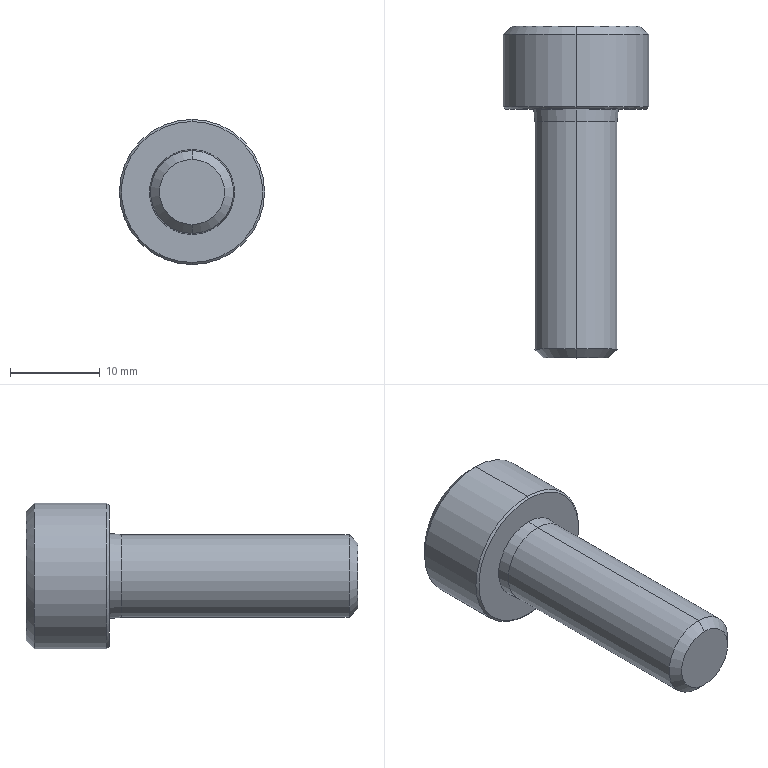Part | SolidWorks | features BaseBody 1 | 1 solid | 36 faces | box 16.154 x 36.923 x 16.154 mm | volume 3494 mm3 | cone 17 | plane 15 | cylinder 4 | commonest cylinder face diameters 9.231 x2 16.154 x2
STEP:
#1=CARTESIAN_POINT('',(-35.061,271.722,102.846));
#2=VERTEX_POINT('',#1);
#3=CARTESIAN_POINT('',(-35.061,271.722,93.615));
#4=VERTEX_POINT('',#3);
#5=CARTESIAN_POINT('',(-35.061,271.722,98.231));
#6=DIRECTION('',(0.,1.,0.));
#7=DIRECTION('',(0.,0.,1.));
#8=AXIS2_PLACEMENT_3D('',#5,#6,#7);
#9=CIRCLE('',#8,4.615);
#10=EDGE_CURVE('',#2,#4,#9,.T.);
#11=ORIENTED_EDGE('',*,*,#10,.T.);
#12=CARTESIAN_POINT('',(-35.061,297.039,93.615));
#13=VERTEX_POINT('',#12);
#14=CARTESIAN_POINT('',(-35.061,270.731,93.615));
#15=DIRECTION('',(0.,1.,0.));
#16=VECTOR('',#15,1000.);
#17=LINE('',#14,#16);
#18=EDGE_CURVE('',#4,#13,#17,.T.);
#19=ORIENTED_EDGE('',*,*,#18,.T.);
#20=CARTESIAN_POINT('',(-35.061,297.039,102.846));
#21=VERTEX_POINT('',#20);
#22=CARTESIAN_POINT('',(-35.061,297.039,98.231));
#23=DIRECTION('',(0.,-1.,0.));
#24=DIRECTION('',(0.,0.,1.));
#25=AXIS2_PLACEMENT_3D('',#22,#23,#24);
#26=CIRCLE('',#25,4.615);
#27=EDGE_CURVE('',#13,#21,#26,.T.);
#28=ORIENTED_EDGE('',*,*,#27,.T.);
#29=CARTESIAN_POINT('',(-35.061,270.731,102.846));
#30=DIRECTION('',(0.,1.,0.));
#31=VECTOR('',#30,1000.);
#32=LINE('',#29,#31);
#33=EDGE_CURVE('',#2,#21,#32,.T.);
#34=ORIENTED_EDGE('',*,*,#33,.F.);
#35=EDGE_LOOP('',(#11,#19,#28,#34));
#36=FACE_OUTER_BOUND('',#35,.T.);
#37=CARTESIAN_POINT('',(-35.061,270.731,98.231));
#38=DIRECTION('',(0.,1.,0.));
#39=DIRECTION('',(0.,0.,1.));
#40=AXIS2_PLACEMENT_3D('',#37,#38,#39);
#41=CYLINDRICAL_SURFACE('',#40,4.615);
#42=ADVANCED_FACE('',(#36),#41,.T.);
#43=CARTESIAN_POINT('',(-35.061,270.731,101.855));
#44=VERTEX_POINT('',#43);
#45=CARTESIAN_POINT('',(-35.061,270.731,94.607));
#46=VERTEX_POINT('',#45);
#47=CARTESIAN_POINT('',(-35.061,270.731,98.231));
#48=DIRECTION('',(0.,1.,0.));
#49=DIRECTION('',(0.,0.,1.));
#50=AXIS2_PLACEMENT_3D('',#47,#48,#49);
#51=CIRCLE('',#50,3.624);
#52=EDGE_CURVE('',#44,#46,#51,.T.);
#53=ORIENTED_EDGE('',*,*,#52,.T.);
#54=CARTESIAN_POINT('',(-35.061,271.722,93.615));
#55=DIRECTION('',(0.,0.7071,-0.7071));
#56=VECTOR('',#55,1000.);
#57=LINE('',#54,#56);
#58=EDGE_CURVE('',#46,#4,#57,.T.);
#59=ORIENTED_EDGE('',*,*,#58,.T.);
#60=ORIENTED_EDGE('',*,*,#10,.F.);
#61=CARTESIAN_POINT('',(-35.061,271.722,102.846));
#62=DIRECTION('',(0.,0.7071,0.7071));
#63=VECTOR('',#62,1000.);
#64=LINE('',#61,#63);
#65=EDGE_CURVE('',#44,#2,#64,.T.);
#66=ORIENTED_EDGE('',*,*,#65,.F.);
#67=EDGE_LOOP('',(#53,#59,#60,#66));
#68=FACE_OUTER_BOUND('',#67,.T.);
#69=CARTESIAN_POINT('',(-35.061,271.722,98.231));
#70=DIRECTION('',(0.,1.,0.));
#71=DIRECTION('',(0.,0.,1.));
#72=AXIS2_PLACEMENT_3D('',#69,#70,#71);
#73=CONICAL_SURFACE('',#72,4.615,0.7854);
#74=ADVANCED_FACE('',(#68),#73,.T.);
#75=ORIENTED_EDGE('',*,*,#27,.F.);
#76=CARTESIAN_POINT('',(-35.061,298.423,93.5));
#77=VERTEX_POINT('',#76);
#78=CARTESIAN_POINT('',(-35.061,298.423,93.5));
#79=DIRECTION('',(0.,0.9965,-0.08305));
#80=VECTOR('',#79,1000.);
#81=LINE('',#78,#80);
#82=EDGE_CURVE('',#13,#77,#81,.T.);
#83=ORIENTED_EDGE('',*,*,#82,.T.);
#84=CARTESIAN_POINT('',(-35.061,298.423,102.962));
#85=VERTEX_POINT('',#84);
#86=CARTESIAN_POINT('',(-35.061,298.423,98.231));
#87=DIRECTION('',(0.,-1.,0.));
#88=DIRECTION('',(0.,0.,1.));
#89=AXIS2_PLACEMENT_3D('',#86,#87,#88);
#90=CIRCLE('',#89,4.731);
#91=EDGE_CURVE('',#77,#85,#90,.T.);
#92=ORIENTED_EDGE('',*,*,#91,.T.);
#93=CARTESIAN_POINT('',(-35.061,298.423,102.962));
#94=DIRECTION('',(0.,0.9965,0.08305));
#95=VECTOR('',#94,1000.);
#96=LINE('',#93,#95);
#97=EDGE_CURVE('',#21,#85,#96,.T.);
#98=ORIENTED_EDGE('',*,*,#97,.F.);
#99=EDGE_LOOP('',(#75,#83,#92,#98));
#100=FACE_OUTER_BOUND('',#99,.T.);
#101=CARTESIAN_POINT('',(-35.061,298.423,98.231));
#102=DIRECTION('',(0.,1.,0.));
#103=DIRECTION('',(0.,0.,1.));
#104=AXIS2_PLACEMENT_3D('',#101,#102,#103);
#105=CONICAL_SURFACE('',#104,4.731,0.08314);
#106=ADVANCED_FACE('',(#100),#105,.T.);
#107=CARTESIAN_POINT('',(-35.061,298.423,106.077));
#108=VERTEX_POINT('',#107);
#109=CARTESIAN_POINT('',(-35.061,298.423,90.385));
#110=VERTEX_POINT('',#109);
#111=CARTESIAN_POINT('',(-35.061,298.423,98.231));
#112=DIRECTION('',(0.,1.,0.));
#113=DIRECTION('',(0.,0.,1.));
#114=AXIS2_PLACEMENT_3D('',#111,#112,#113);
#115=CIRCLE('',#114,7.846);
#116=EDGE_CURVE('',#108,#110,#115,.T.);
#117=ORIENTED_EDGE('',*,*,#116,.T.);
#118=CARTESIAN_POINT('',(-35.061,298.654,90.154));
#119=VERTEX_POINT('',#118);
#120=CARTESIAN_POINT('',(-35.061,298.654,90.154));
#121=DIRECTION('',(0.,0.7071,-0.7071));
#122=VECTOR('',#121,1000.);
#123=LINE('',#120,#122);
#124=EDGE_CURVE('',#110,#119,#123,.T.);
#125=ORIENTED_EDGE('',*,*,#124,.T.);
#126=CARTESIAN_POINT('',(-35.061,298.654,106.308));
#127=VERTEX_POINT('',#126);
#128=CARTESIAN_POINT('',(-35.061,298.654,98.231));
#129=DIRECTION('',(0.,-1.,0.));
#130=DIRECTION('',(-1.,0.,0.));
#131=AXIS2_PLACEMENT_3D('',#128,#129,#130);
#132=CIRCLE('',#131,8.077);
#133=EDGE_CURVE('',#119,#127,#132,.T.);
#134=ORIENTED_EDGE('',*,*,#133,.T.);
#135=CARTESIAN_POINT('',(-35.061,298.654,106.308));
#136=DIRECTION('',(0.,0.7071,0.7071));
#137=VECTOR('',#136,1000.);
#138=LINE('',#135,#137);
#139=EDGE_CURVE('',#108,#127,#138,.T.);
#140=ORIENTED_EDGE('',*,*,#139,.F.);
#141=EDGE_LOOP('',(#117,#125,#134,#140));
#142=FACE_OUTER_BOUND('',#141,.T.);
#143=CARTESIAN_POINT('',(-35.061,298.654,98.231));
#144=DIRECTION('',(0.,1.,0.));
#145=DIRECTION('',(0.,0.,1.));
#146=AXIS2_PLACEMENT_3D('',#143,#144,#145);
#147=CONICAL_SURFACE('',#146,8.077,0.7854);
#148=ADVANCED_FACE('',(#142),#147,.T.);
#149=ORIENTED_EDGE('',*,*,#133,.F.);
#150=CARTESIAN_POINT('',(-35.061,306.731,90.154));
#151=VERTEX_POINT('',#150);
#152=CARTESIAN_POINT('',(-35.061,270.731,90.154));
#153=DIRECTION('',(0.,1.,0.));
#154=VECTOR('',#153,1000.);
#155=LINE('',#152,#154);
#156=EDGE_CURVE('',#119,#151,#155,.T.);
#157=ORIENTED_EDGE('',*,*,#156,.T.);
#158=CARTESIAN_POINT('',(-35.061,306.731,106.308));
#159=VERTEX_POINT('',#158);
#160=CARTESIAN_POINT('',(-35.061,306.731,98.231));
#161=DIRECTION('',(0.,-1.,0.));
#162=DIRECTION('',(0.,0.,1.));
#163=AXIS2_PLACEMENT_3D('',#160,#161,#162);
#164=CIRCLE('',#163,8.077);
#165=EDGE_CURVE('',#151,#159,#164,.T.);
#166=ORIENTED_EDGE('',*,*,#165,.T.);
#167=CARTESIAN_POINT('',(-35.061,270.731,106.308));
#168=DIRECTION('',(0.,1.,0.));
#169=VECTOR('',#168,1000.);
#170=LINE('',#167,#169);
#171=EDGE_CURVE('',#127,#159,#170,.T.);
#172=ORIENTED_EDGE('',*,*,#171,.F.);
#173=EDGE_LOOP('',(#149,#157,#166,#172));
#174=FACE_OUTER_BOUND('',#173,.T.);
#175=CARTESIAN_POINT('',(-35.061,270.731,98.231));
#176=DIRECTION('',(0.,1.,0.));
#177=DIRECTION('',(0.,0.,1.));
#178=AXIS2_PLACEMENT_3D('',#175,#176,#177);
#179=CYLINDRICAL_SURFACE('',#178,8.077);
#180=ADVANCED_FACE('',(#174),#179,.T.);
#181=CARTESIAN_POINT('',(-35.061,307.654,91.077));
#182=VERTEX_POINT('',#181);
#183=CARTESIAN_POINT('',(-35.061,307.654,105.385));
#184=VERTEX_POINT('',#183);
#185=CARTESIAN_POINT('',(-35.061,307.654,98.231));
#186=DIRECTION('',(0.,-1.,0.));
#187=DIRECTION('',(0.,0.,-1.));
#188=AXIS2_PLACEMENT_3D('',#185,#186,#187);
#189=CIRCLE('',#188,7.154);
#190=EDGE_CURVE('',#182,#184,#189,.T.);
#191=ORIENTED_EDGE('',*,*,#190,.T.);
#192=CARTESIAN_POINT('',(-35.061,306.731,106.308));
#193=DIRECTION('',(0.,-0.7071,0.7071));
#194=VECTOR('',#193,1000.);
#195=LINE('',#192,#194);
#196=EDGE_CURVE('',#184,#159,#195,.T.);
#197=ORIENTED_EDGE('',*,*,#196,.T.);
#198=ORIENTED_EDGE('',*,*,#165,.F.);
#199=CARTESIAN_POINT('',(-35.061,306.731,90.154));
#200=DIRECTION('',(0.,-0.7071,-0.7071));
#201=VECTOR('',#200,1000.);
#202=LINE('',#199,#201);
#203=EDGE_CURVE('',#182,#151,#202,.T.);
#204=ORIENTED_EDGE('',*,*,#203,.F.);
#205=EDGE_LOOP('',(#191,#197,#198,#204));
#206=FACE_OUTER_BOUND('',#205,.T.);
#207=CARTESIAN_POINT('',(-35.061,306.731,98.231));
#208=DIRECTION('',(0.,-1.,0.));
#209=DIRECTION('',(0.,0.,-1.));
#210=AXIS2_PLACEMENT_3D('',#207,#208,#209);
#211=CONICAL_SURFACE('',#210,8.077,0.7854);
#212=ADVANCED_FACE('',(#206),#211,.T.);
#213=CARTESIAN_POINT('',(-35.061,307.118,101.692));
#214=VERTEX_POINT('',#213);
#215=CARTESIAN_POINT('',(-33.063,307.654,101.692));
#216=VERTEX_POINT('',#215);
#217=CARTESIAN_POINT('',(-35.061,307.118,101.692));
#218=CARTESIAN_POINT('',(-34.714,307.118,101.692));
#219=CARTESIAN_POINT('',(-34.372,307.172,101.692));
#220=CARTESIAN_POINT('',(-33.698,307.363,101.692));
#221=CARTESIAN_POINT('',(-33.376,307.497,101.692));
#222=CARTESIAN_POINT('',(-33.063,307.654,101.692));
#223=B_SPLINE_CURVE_WITH_KNOTS('',3,(#217,#218,#219,#220,#221,#222),.UNSPECIFIED.,.F.,.F.,(4,2,4),(0.002072,0.0031,0.004129),.UNSPECIFIED.);
#224=EDGE_CURVE('',#214,#216,#223,.T.);
#225=ORIENTED_EDGE('',*,*,#224,.F.);
#226=CARTESIAN_POINT('',(-35.061,307.654,102.228));
#227=VERTEX_POINT('',#226);
#228=CARTESIAN_POINT('',(-35.061,307.654,102.228));
#229=DIRECTION('',(0.,0.7071,0.7071));
#230=VECTOR('',#229,1000.);
#231=LINE('',#228,#230);
#232=EDGE_CURVE('',#214,#227,#231,.T.);
#233=ORIENTED_EDGE('',*,*,#232,.T.);
#234=CARTESIAN_POINT('',(-35.061,307.654,98.231));
#235=DIRECTION('',(0.,1.,0.));
#236=DIRECTION('',(0.,0.,1.));
#237=AXIS2_PLACEMENT_3D('',#234,#235,#236);
#238=CIRCLE('',#237,3.997);
#239=EDGE_CURVE('',#227,#216,#238,.T.);
#240=ORIENTED_EDGE('',*,*,#239,.T.);
#241=EDGE_LOOP('',(#225,#233,#240));
#242=FACE_OUTER_BOUND('',#241,.T.);
#243=CARTESIAN_POINT('',(-35.061,307.654,98.231));
#244=DIRECTION('',(0.,1.,0.));
#245=DIRECTION('',(0.,0.,1.));
#246=AXIS2_PLACEMENT_3D('',#243,#244,#245);
#247=CONICAL_SURFACE('',#246,3.997,0.7854);
#248=ADVANCED_FACE('',(#242),#247,.F.);
#249=CARTESIAN_POINT('',(-35.061,301.04,98.231));
#250=VERTEX_POINT('',#249);
#251=CARTESIAN_POINT('',(-35.061,303.039,101.692));
#252=VERTEX_POINT('',#251);
#253=CARTESIAN_POINT('',(-35.061,303.039,101.692));
#254=DIRECTION('',(0.,0.5,0.866));
#255=VECTOR('',#254,1000.);
#256=LINE('',#253,#255);
#257=EDGE_CURVE('',#250,#252,#256,.T.);
#258=ORIENTED_EDGE('',*,*,#257,.F.);
#259=CARTESIAN_POINT('',(-35.061,303.039,94.769));
#260=VERTEX_POINT('',#259);
#261=CARTESIAN_POINT('',(-35.061,303.039,94.769));
#262=DIRECTION('',(0.,0.5,-0.866));
#263=VECTOR('',#262,1000.);
#264=LINE('',#261,#263);
#265=EDGE_CURVE('',#250,#260,#264,.T.);
#266=ORIENTED_EDGE('',*,*,#265,.T.);
#267=CARTESIAN_POINT('',(-38.059,303.039,96.5));
#268=VERTEX_POINT('',#267);
#269=CARTESIAN_POINT('',(-35.061,303.039,98.231));
#270=DIRECTION('',(0.,-1.,0.));
#271=DIRECTION('',(0.,0.,1.));
#272=AXIS2_PLACEMENT_3D('',#269,#270,#271);
#273=CIRCLE('',#272,3.462);
#274=EDGE_CURVE('',#268,#260,#273,.T.);
#275=ORIENTED_EDGE('',*,*,#274,.F.);
#276=CARTESIAN_POINT('',(-38.059,303.039,99.962));
#277=VERTEX_POINT('',#276);
#278=CARTESIAN_POINT('',(-35.061,303.039,98.231));
#279=DIRECTION('',(0.,-1.,0.));
#280=DIRECTION('',(0.,0.,1.));
#281=AXIS2_PLACEMENT_3D('',#278,#279,#280);
#282=CIRCLE('',#281,3.462);
#283=EDGE_CURVE('',#277,#268,#282,.T.);
#284=ORIENTED_EDGE('',*,*,#283,.F.);
#285=CARTESIAN_POINT('',(-35.061,303.039,98.231));
#286=DIRECTION('',(0.,-1.,0.));
#287=DIRECTION('',(0.,0.,1.));
#288=AXIS2_PLACEMENT_3D('',#285,#286,#287);
#289=CIRCLE('',#288,3.462);
#290=EDGE_CURVE('',#252,#277,#289,.T.);
#291=ORIENTED_EDGE('',*,*,#290,.F.);
#292=EDGE_LOOP('',(#258,#266,#275,#284,#291));
#293=FACE_OUTER_BOUND('',#292,.T.);
#294=CARTESIAN_POINT('',(-35.061,303.039,98.231));
#295=DIRECTION('',(0.,1.,0.));
#296=DIRECTION('',(0.,0.,1.));
#297=AXIS2_PLACEMENT_3D('',#294,#295,#296);
#298=CONICAL_SURFACE('',#297,3.462,1.047);
#299=ADVANCED_FACE('',(#293),#298,.F.);
#300=ORIENTED_EDGE('',*,*,#18,.F.);
#301=CARTESIAN_POINT('',(-35.061,271.722,98.231));
#302=DIRECTION('',(0.,1.,0.));
#303=DIRECTION('',(0.,0.,1.));
#304=AXIS2_PLACEMENT_3D('',#301,#302,#303);
#305=CIRCLE('',#304,4.615);
#306=EDGE_CURVE('',#4,#2,#305,.T.);
#307=ORIENTED_EDGE('',*,*,#306,.T.);
#308=ORIENTED_EDGE('',*,*,#33,.T.);
#309=CARTESIAN_POINT('',(-35.061,297.039,98.231));
#310=DIRECTION('',(0.,-1.,0.));
#311=DIRECTION('',(0.,0.,1.));
#312=AXIS2_PLACEMENT_3D('',#309,#310,#311);
#313=CIRCLE('',#312,4.615);
#314=EDGE_CURVE('',#21,#13,#313,.T.);
#315=ORIENTED_EDGE('',*,*,#314,.T.);
#316=EDGE_LOOP('',(#300,#307,#308,#315));
#317=FACE_OUTER_BOUND('',#316,.T.);
#318=CARTESIAN_POINT('',(-35.061,270.731,98.231));
#319=DIRECTION('',(0.,1.,0.));
#320=DIRECTION('',(0.,0.,1.));
#321=AXIS2_PLACEMENT_3D('',#318,#319,#320);
#322=CYLINDRICAL_SURFACE('',#321,4.615);
#323=ADVANCED_FACE('',(#317),#322,.T.);
#324=ORIENTED_EDGE('',*,*,#58,.F.);
#325=CARTESIAN_POINT('',(-35.061,270.731,98.231));
#326=DIRECTION('',(0.,1.,0.));
#327=DIRECTION('',(0.,0.,1.));
#328=AXIS2_PLACEMENT_3D('',#325,#326,#327);
#329=CIRCLE('',#328,3.624);
#330=EDGE_CURVE('',#46,#44,#329,.T.);
#331=ORIENTED_EDGE('',*,*,#330,.T.);
#332=ORIENTED_EDGE('',*,*,#65,.T.);
#333=ORIENTED_EDGE('',*,*,#306,.F.);
#334=EDGE_LOOP('',(#324,#331,#332,#333));
#335=FACE_OUTER_BOUND('',#334,.T.);
#336=CARTESIAN_POINT('',(-35.061,271.722,98.231));
#337=DIRECTION('',(0.,1.,0.));
#338=DIRECTION('',(0.,0.,1.));
#339=AXIS2_PLACEMENT_3D('',#336,#337,#338);
#340=CONICAL_SURFACE('',#339,4.615,0.7854);
#341=ADVANCED_FACE('',(#335),#340,.T.);
#342=ORIENTED_EDGE('',*,*,#82,.F.);
#343=ORIENTED_EDGE('',*,*,#314,.F.);
#344=ORIENTED_EDGE('',*,*,#97,.T.);
#345=CARTESIAN_POINT('',(-35.061,298.423,98.231));
#346=DIRECTION('',(0.,-1.,0.));
#347=DIRECTION('',(0.,0.,1.));
#348=AXIS2_PLACEMENT_3D('',#345,#346,#347);
#349=CIRCLE('',#348,4.731);
#350=EDGE_CURVE('',#85,#77,#349,.T.);
#351=ORIENTED_EDGE('',*,*,#350,.T.);
#352=EDGE_LOOP('',(#342,#343,#344,#351));
#353=FACE_OUTER_BOUND('',#352,.T.);
#354=CARTESIAN_POINT('',(-35.061,298.423,98.231));
#355=DIRECTION('',(0.,1.,0.));
#356=DIRECTION('',(0.,0.,1.));
#357=AXIS2_PLACEMENT_3D('',#354,#355,#356);
#358=CONICAL_SURFACE('',#357,4.731,0.08314);
#359=ADVANCED_FACE('',(#353),#358,.T.);
#360=ORIENTED_EDGE('',*,*,#52,.F.);
#361=ORIENTED_EDGE('',*,*,#330,.F.);
#362=EDGE_LOOP('',(#360,#361));
#363=FACE_OUTER_BOUND('',#362,.T.);
#364=CARTESIAN_POINT('',(-35.061,270.731,94.607));
#365=DIRECTION('',(0.,1.,0.));
#366=DIRECTION('',(0.,0.,1.));
#367=AXIS2_PLACEMENT_3D('',#364,#365,#366);
#368=PLANE('',#367);
#369=ADVANCED_FACE('',(#363),#368,.F.);
#370=ORIENTED_EDGE('',*,*,#350,.F.);
#371=ORIENTED_EDGE('',*,*,#91,.F.);
#372=EDGE_LOOP('',(#370,#371));
#373=FACE_BOUND('',#372,.T.);
#374=ORIENTED_EDGE('',*,*,#116,.F.);
#375=CARTESIAN_POINT('',(-35.061,298.423,98.231));
#376=DIRECTION('',(0.,1.,0.));
#377=DIRECTION('',(0.,0.,1.));
#378=AXIS2_PLACEMENT_3D('',#375,#376,#377);
#379=CIRCLE('',#378,7.846);
#380=EDGE_CURVE('',#110,#108,#379,.T.);
#381=ORIENTED_EDGE('',*,*,#380,.F.);
#382=EDGE_LOOP('',(#374,#381));
#383=FACE_OUTER_BOUND('',#382,.T.);
#384=CARTESIAN_POINT('',(-35.061,298.423,90.385));
#385=DIRECTION('',(0.,1.,0.));
#386=DIRECTION('',(0.,0.,1.));
#387=AXIS2_PLACEMENT_3D('',#384,#385,#386);
#388=PLANE('',#387);
#389=ADVANCED_FACE('',(#373,#383),#388,.F.);
#390=ORIENTED_EDGE('',*,*,#124,.F.);
#391=ORIENTED_EDGE('',*,*,#380,.T.);
#392=ORIENTED_EDGE('',*,*,#139,.T.);
#393=CARTESIAN_POINT('',(-35.061,298.654,98.231));
#394=DIRECTION('',(0.,-1.,0.));
#395=DIRECTION('',(-1.,0.,0.));
#396=AXIS2_PLACEMENT_3D('',#393,#394,#395);
#397=CIRCLE('',#396,8.077);
#398=EDGE_CURVE('',#127,#119,#397,.T.);
#399=ORIENTED_EDGE('',*,*,#398,.T.);
#400=EDGE_LOOP('',(#390,#391,#392,#399));
#401=FACE_OUTER_BOUND('',#400,.T.);
#402=CARTESIAN_POINT('',(-35.061,298.654,98.231));
#403=DIRECTION('',(0.,1.,0.));
#404=DIRECTION('',(0.,0.,1.));
#405=AXIS2_PLACEMENT_3D('',#402,#403,#404);
#406=CONICAL_SURFACE('',#405,8.077,0.7854);
#407=ADVANCED_FACE('',(#401),#406,.T.);
#408=ORIENTED_EDGE('',*,*,#156,.F.);
#409=ORIENTED_EDGE('',*,*,#398,.F.);
#410=ORIENTED_EDGE('',*,*,#171,.T.);
#411=CARTESIAN_POINT('',(-35.061,306.731,98.231));
#412=DIRECTION('',(0.,-1.,0.));
#413=DIRECTION('',(0.,0.,1.));
#414=AXIS2_PLACEMENT_3D('',#411,#412,#413);
#415=CIRCLE('',#414,8.077);
#416=EDGE_CURVE('',#159,#151,#415,.T.);
#417=ORIENTED_EDGE('',*,*,#416,.T.);
#418=EDGE_LOOP('',(#408,#409,#410,#417));
#419=FACE_OUTER_BOUND('',#418,.T.);
#420=CARTESIAN_POINT('',(-35.061,270.731,98.231));
#421=DIRECTION('',(0.,1.,0.));
#422=DIRECTION('',(0.,0.,1.));
#423=AXIS2_PLACEMENT_3D('',#420,#421,#422);
#424=CYLINDRICAL_SURFACE('',#423,8.077);
#425=ADVANCED_FACE('',(#419),#424,.T.);
#426=ORIENTED_EDGE('',*,*,#196,.F.);
#427=CARTESIAN_POINT('',(-35.061,307.654,98.231));
#428=DIRECTION('',(0.,-1.,0.));
#429=DIRECTION('',(0.,0.,-1.));
#430=AXIS2_PLACEMENT_3D('',#427,#428,#429);
#431=CIRCLE('',#430,7.154);
#432=EDGE_CURVE('',#184,#182,#431,.T.);
#433=ORIENTED_EDGE('',*,*,#432,.T.);
#434=ORIENTED_EDGE('',*,*,#203,.T.);
#435=ORIENTED_EDGE('',*,*,#416,.F.);
#436=EDGE_LOOP('',(#426,#433,#434,#435));
#437=FACE_OUTER_BOUND('',#436,.T.);
#438=CARTESIAN_POINT('',(-35.061,306.731,98.231));
#439=DIRECTION('',(0.,-1.,0.));
#440=DIRECTION('',(0.,0.,-1.));
#441=AXIS2_PLACEMENT_3D('',#438,#439,#440);
#442=CONICAL_SURFACE('',#441,8.077,0.7854);
#443=ADVANCED_FACE('',(#437),#442,.T.);
#444=CARTESIAN_POINT('',(-31.064,307.654,98.231));
#445=VERTEX_POINT('',#444);
#446=CARTESIAN_POINT('',(-35.061,307.654,98.231));
#447=DIRECTION('',(0.,1.,0.));
#448=DIRECTION('',(0.,0.,1.));
#449=AXIS2_PLACEMENT_3D('',#446,#447,#448);
#450=CIRCLE('',#449,3.997);
#451=EDGE_CURVE('',#216,#445,#450,.T.);
#452=ORIENTED_EDGE('',*,*,#451,.F.);
#453=ORIENTED_EDGE('',*,*,#239,.F.);
#454=CARTESIAN_POINT('',(-37.06,307.654,101.692));
#455=VERTEX_POINT('',#454);
#456=CARTESIAN_POINT('',(-35.061,307.654,98.231));
#457=DIRECTION('',(0.,1.,0.));
#458=DIRECTION('',(0.,0.,1.));
#459=AXIS2_PLACEMENT_3D('',#456,#457,#458);
#460=CIRCLE('',#459,3.997);
#461=EDGE_CURVE('',#455,#227,#460,.T.);
#462=ORIENTED_EDGE('',*,*,#461,.F.);
#463=CARTESIAN_POINT('',(-39.058,307.654,98.231));
#464=VERTEX_POINT('',#463);
#465=CARTESIAN_POINT('',(-35.061,307.654,98.231));
#466=DIRECTION('',(0.,1.,0.));
#467=DIRECTION('',(0.,0.,1.));
#468=AXIS2_PLACEMENT_3D('',#465,#466,#467);
#469=CIRCLE('',#468,3.997);
#470=EDGE_CURVE('',#464,#455,#469,.T.);
#471=ORIENTED_EDGE('',*,*,#470,.F.);
#472=CARTESIAN_POINT('',(-37.06,307.654,94.769));
#473=VERTEX_POINT('',#472);
#474=CARTESIAN_POINT('',(-35.061,307.654,98.231));
#475=DIRECTION('',(0.,1.,0.));
#476=DIRECTION('',(0.,0.,1.));
#477=AXIS2_PLACEMENT_3D('',#474,#475,#476);
#478=CIRCLE('',#477,3.997);
#479=EDGE_CURVE('',#473,#464,#478,.T.);
#480=ORIENTED_EDGE('',*,*,#479,.F.);
#481=CARTESIAN_POINT('',(-33.063,307.654,94.769));
#482=VERTEX_POINT('',#481);
#483=CARTESIAN_POINT('',(-35.061,307.654,98.231));
#484=DIRECTION('',(0.,1.,0.));
#485=DIRECTION('',(0.,0.,1.));
#486=AXIS2_PLACEMENT_3D('',#483,#484,#485);
#487=CIRCLE('',#486,3.997);
#488=EDGE_CURVE('',#482,#473,#487,.T.);
#489=ORIENTED_EDGE('',*,*,#488,.F.);
#490=CARTESIAN_POINT('',(-35.061,307.654,98.231));
#491=DIRECTION('',(0.,1.,0.));
#492=DIRECTION('',(0.,0.,1.));
#493=AXIS2_PLACEMENT_3D('',#490,#491,#492);
#494=CIRCLE('',#493,3.997);
#495=EDGE_CURVE('',#445,#482,#494,.T.);
#496=ORIENTED_EDGE('',*,*,#495,.F.);
#497=EDGE_LOOP('',(#452,#453,#462,#471,#480,#489,#496));
#498=FACE_BOUND('',#497,.T.);
#499=ORIENTED_EDGE('',*,*,#190,.F.);
#500=ORIENTED_EDGE('',*,*,#432,.F.);
#501=EDGE_LOOP('',(#499,#500));
#502=FACE_OUTER_BOUND('',#501,.T.);
#503=CARTESIAN_POINT('',(-35.061,307.654,94.234));
#504=DIRECTION('',(0.,-1.,0.));
#505=DIRECTION('',(0.,0.,-1.));
#506=AXIS2_PLACEMENT_3D('',#503,#504,#505);
#507=PLANE('',#506);
#508=ADVANCED_FACE('',(#498,#502),#507,.F.);
#509=CARTESIAN_POINT('',(-31.064,307.654,98.231));
#510=CARTESIAN_POINT('',(-31.22,307.498,97.96));
#511=CARTESIAN_POINT('',(-31.38,307.365,97.684));
#512=CARTESIAN_POINT('',(-31.628,307.223,97.254));
#513=CARTESIAN_POINT('',(-31.712,307.185,97.108));
#514=CARTESIAN_POINT('',(-31.884,307.133,96.811));
#515=CARTESIAN_POINT('',(-31.972,307.119,96.657));
#516=CARTESIAN_POINT('',(-32.234,307.118,96.204));
#517=CARTESIAN_POINT('',(-32.406,307.17,95.907));
#518=CARTESIAN_POINT('',(-32.744,307.362,95.321));
#519=CARTESIAN_POINT('',(-32.906,307.497,95.041));
#520=CARTESIAN_POINT('',(-33.063,307.654,94.769));
#521=B_SPLINE_CURVE_WITH_KNOTS('',3,(#509,#510,#511,#512,#513,#514,#515,#516,#517,#518,#519,#520),.UNSPECIFIED.,.F.,.F.,(4,2,2,2,2,4),(0.,0.001032,0.001548,0.002064,0.003097,0.004129),.UNSPECIFIED.);
#522=EDGE_CURVE('',#445,#482,#521,.T.);
#523=ORIENTED_EDGE('',*,*,#522,.F.);
#524=ORIENTED_EDGE('',*,*,#495,.T.);
#525=EDGE_LOOP('',(#523,#524));
#526=FACE_OUTER_BOUND('',#525,.T.);
#527=CARTESIAN_POINT('',(-35.061,307.654,98.231));
#528=DIRECTION('',(0.,1.,0.));
#529=DIRECTION('',(0.,0.,1.));
#530=AXIS2_PLACEMENT_3D('',#527,#528,#529);
#531=CONICAL_SURFACE('',#530,3.997,0.7854);
#532=ADVANCED_FACE('',(#526),#531,.F.);
#533=CARTESIAN_POINT('',(-33.063,307.654,101.692));
#534=CARTESIAN_POINT('',(-32.906,307.498,101.422));
#535=CARTESIAN_POINT('',(-32.747,307.365,101.145));
#536=CARTESIAN_POINT('',(-32.499,307.223,100.716));
#537=CARTESIAN_POINT('',(-32.415,307.185,100.57));
#538=CARTESIAN_POINT('',(-32.243,307.133,100.272));
#539=CARTESIAN_POINT('',(-32.154,307.119,100.119));
#540=CARTESIAN_POINT('',(-31.893,307.118,99.666));
#541=CARTESIAN_POINT('',(-31.721,307.17,99.369));
#542=CARTESIAN_POINT('',(-31.383,307.362,98.783));
#543=CARTESIAN_POINT('',(-31.221,307.497,98.503));
#544=CARTESIAN_POINT('',(-31.064,307.654,98.231));
#545=B_SPLINE_CURVE_WITH_KNOTS('',3,(#533,#534,#535,#536,#537,#538,#539,#540,#541,#542,#543,#544),.UNSPECIFIED.,.F.,.F.,(4,2,2,2,2,4),(0.,0.001032,0.001548,0.002064,0.003097,0.004129),.UNSPECIFIED.);
#546=EDGE_CURVE('',#216,#445,#545,.T.);
#547=ORIENTED_EDGE('',*,*,#546,.F.);
#548=ORIENTED_EDGE('',*,*,#451,.T.);
#549=EDGE_LOOP('',(#547,#548));
#550=FACE_OUTER_BOUND('',#549,.T.);
#551=CARTESIAN_POINT('',(-35.061,307.654,98.231));
#552=DIRECTION('',(0.,1.,0.));
#553=DIRECTION('',(0.,0.,1.));
#554=AXIS2_PLACEMENT_3D('',#551,#552,#553);
#555=CONICAL_SURFACE('',#554,3.997,0.7854);
#556=ADVANCED_FACE('',(#550),#555,.F.);
#557=ORIENTED_EDGE('',*,*,#232,.F.);
#558=CARTESIAN_POINT('',(-37.06,307.654,101.692));
#559=CARTESIAN_POINT('',(-36.746,307.497,101.692));
#560=CARTESIAN_POINT('',(-36.426,307.364,101.692));
#561=CARTESIAN_POINT('',(-35.928,307.222,101.692));
#562=CARTESIAN_POINT('',(-35.759,307.184,101.692));
#563=CARTESIAN_POINT('',(-35.414,307.132,101.692));
#564=CARTESIAN_POINT('',(-35.236,307.118,101.692));
#565=CARTESIAN_POINT('',(-35.061,307.118,101.692));
#566=B_SPLINE_CURVE_WITH_KNOTS('',3,(#558,#559,#560,#561,#562,#563,#564,#565),.UNSPECIFIED.,.F.,.F.,(4,2,2,4),(0.,0.001036,0.001554,0.002072),.UNSPECIFIED.);
#567=EDGE_CURVE('',#455,#214,#566,.T.);
#568=ORIENTED_EDGE('',*,*,#567,.F.);
#569=ORIENTED_EDGE('',*,*,#461,.T.);
#570=EDGE_LOOP('',(#557,#568,#569));
#571=FACE_OUTER_BOUND('',#570,.T.);
#572=CARTESIAN_POINT('',(-35.061,307.654,98.231));
#573=DIRECTION('',(0.,1.,0.));
#574=DIRECTION('',(0.,0.,1.));
#575=AXIS2_PLACEMENT_3D('',#572,#573,#574);
#576=CONICAL_SURFACE('',#575,3.997,0.7854);
#577=ADVANCED_FACE('',(#571),#576,.F.);
#578=CARTESIAN_POINT('',(-39.058,307.654,98.231));
#579=CARTESIAN_POINT('',(-38.902,307.498,98.501));
#580=CARTESIAN_POINT('',(-38.742,307.365,98.778));
#581=CARTESIAN_POINT('',(-38.494,307.223,99.207));
#582=CARTESIAN_POINT('',(-38.41,307.185,99.353));
#583=CARTESIAN_POINT('',(-38.238,307.133,99.651));
#584=CARTESIAN_POINT('',(-38.15,307.119,99.804));
#585=CARTESIAN_POINT('',(-37.888,307.118,100.257));
#586=CARTESIAN_POINT('',(-37.717,307.17,100.554));
#587=CARTESIAN_POINT('',(-37.378,307.362,101.14));
#588=CARTESIAN_POINT('',(-37.217,307.497,101.42));
#589=CARTESIAN_POINT('',(-37.06,307.654,101.692));
#590=B_SPLINE_CURVE_WITH_KNOTS('',3,(#578,#579,#580,#581,#582,#583,#584,#585,#586,#587,#588,#589),.UNSPECIFIED.,.F.,.F.,(4,2,2,2,2,4),(0.,0.001032,0.001548,0.002064,0.003097,0.004129),.UNSPECIFIED.);
#591=EDGE_CURVE('',#464,#455,#590,.T.);
#592=ORIENTED_EDGE('',*,*,#591,.F.);
#593=ORIENTED_EDGE('',*,*,#470,.T.);
#594=EDGE_LOOP('',(#592,#593));
#595=FACE_OUTER_BOUND('',#594,.T.);
#596=CARTESIAN_POINT('',(-35.061,307.654,98.231));
#597=DIRECTION('',(0.,1.,0.));
#598=DIRECTION('',(0.,0.,1.));
#599=AXIS2_PLACEMENT_3D('',#596,#597,#598);
#600=CONICAL_SURFACE('',#599,3.997,0.7854);
#601=ADVANCED_FACE('',(#595),#600,.F.);
#602=CARTESIAN_POINT('',(-37.06,307.654,94.769));
#603=CARTESIAN_POINT('',(-37.216,307.498,95.04));
#604=CARTESIAN_POINT('',(-37.376,307.365,95.316));
#605=CARTESIAN_POINT('',(-37.624,307.223,95.746));
#606=CARTESIAN_POINT('',(-37.708,307.185,95.892));
#607=CARTESIAN_POINT('',(-37.88,307.133,96.189));
#608=CARTESIAN_POINT('',(-37.968,307.119,96.343));
#609=CARTESIAN_POINT('',(-38.23,307.118,96.796));
#610=CARTESIAN_POINT('',(-38.401,307.17,97.093));
#611=CARTESIAN_POINT('',(-38.739,307.362,97.679));
#612=CARTESIAN_POINT('',(-38.901,307.497,97.959));
#613=CARTESIAN_POINT('',(-39.058,307.654,98.231));
#614=B_SPLINE_CURVE_WITH_KNOTS('',3,(#602,#603,#604,#605,#606,#607,#608,#609,#610,#611,#612,#613),.UNSPECIFIED.,.F.,.F.,(4,2,2,2,2,4),(0.,0.001032,0.001548,0.002064,0.003097,0.004129),.UNSPECIFIED.);
#615=EDGE_CURVE('',#473,#464,#614,.T.);
#616=ORIENTED_EDGE('',*,*,#615,.F.);
#617=ORIENTED_EDGE('',*,*,#479,.T.);
#618=EDGE_LOOP('',(#616,#617));
#619=FACE_OUTER_BOUND('',#618,.T.);
#620=CARTESIAN_POINT('',(-35.061,307.654,98.231));
#621=DIRECTION('',(0.,1.,0.));
#622=DIRECTION('',(0.,0.,1.));
#623=AXIS2_PLACEMENT_3D('',#620,#621,#622);
#624=CONICAL_SURFACE('',#623,3.997,0.7854);
#625=ADVANCED_FACE('',(#619),#624,.F.);
#626=CARTESIAN_POINT('',(-33.063,307.654,94.769));
#627=CARTESIAN_POINT('',(-33.375,307.498,94.769));
#628=CARTESIAN_POINT('',(-33.694,307.365,94.769));
#629=CARTESIAN_POINT('',(-34.19,307.223,94.769));
#630=CARTESIAN_POINT('',(-34.359,307.185,94.769));
#631=CARTESIAN_POINT('',(-34.702,307.133,94.769));
#632=CARTESIAN_POINT('',(-34.879,307.119,94.769));
#633=CARTESIAN_POINT('',(-35.403,307.118,94.769));
#634=CARTESIAN_POINT('',(-35.746,307.17,94.769));
#635=CARTESIAN_POINT('',(-36.422,307.362,94.769));
#636=CARTESIAN_POINT('',(-36.746,307.497,94.769));
#637=CARTESIAN_POINT('',(-37.06,307.654,94.769));
#638=B_SPLINE_CURVE_WITH_KNOTS('',3,(#626,#627,#628,#629,#630,#631,#632,#633,#634,#635,#636,#637),.UNSPECIFIED.,.F.,.F.,(4,2,2,2,2,4),(0.,0.001032,0.001548,0.002064,0.003097,0.004129),.UNSPECIFIED.);
#639=EDGE_CURVE('',#482,#473,#638,.T.);
#640=ORIENTED_EDGE('',*,*,#639,.F.);
#641=ORIENTED_EDGE('',*,*,#488,.T.);
#642=EDGE_LOOP('',(#640,#641));
#643=FACE_OUTER_BOUND('',#642,.T.);
#644=CARTESIAN_POINT('',(-35.061,307.654,98.231));
#645=DIRECTION('',(0.,1.,0.));
#646=DIRECTION('',(0.,0.,1.));
#647=AXIS2_PLACEMENT_3D('',#644,#645,#646);
#648=CONICAL_SURFACE('',#647,3.997,0.7854);
#649=ADVANCED_FACE('',(#643),#648,.F.);
#650=CARTESIAN_POINT('',(-33.063,303.039,94.769));
#651=VERTEX_POINT('',#650);
#652=CARTESIAN_POINT('',(-33.063,303.039,94.769));
#653=DIRECTION('',(0.,1.,0.));
#654=VECTOR('',#653,1000.);
#655=LINE('',#652,#654);
#656=EDGE_CURVE('',#651,#482,#655,.T.);
#657=ORIENTED_EDGE('',*,*,#656,.F.);
#658=CARTESIAN_POINT('',(-32.063,303.039,96.5));
#659=VERTEX_POINT('',#658);
#660=CARTESIAN_POINT('',(-31.064,303.039,98.231));
#661=DIRECTION('',(-0.5,0.,-0.866));
#662=VECTOR('',#661,1000.);
#663=LINE('',#660,#662);
#664=EDGE_CURVE('',#659,#651,#663,.T.);
#665=ORIENTED_EDGE('',*,*,#664,.F.);
#666=CARTESIAN_POINT('',(-31.064,303.039,98.231));
#667=VERTEX_POINT('',#666);
#668=CARTESIAN_POINT('',(-31.064,303.039,98.231));
#669=DIRECTION('',(-0.5,0.,-0.866));
#670=VECTOR('',#669,1000.);
#671=LINE('',#668,#670);
#672=EDGE_CURVE('',#667,#659,#671,.T.);
#673=ORIENTED_EDGE('',*,*,#672,.F.);
#674=CARTESIAN_POINT('',(-31.064,303.039,98.231));
#675=DIRECTION('',(0.,-1.,0.));
#676=VECTOR('',#675,1000.);
#677=LINE('',#674,#676);
#678=EDGE_CURVE('',#445,#667,#677,.T.);
#679=ORIENTED_EDGE('',*,*,#678,.F.);
#680=ORIENTED_EDGE('',*,*,#522,.T.);
#681=EDGE_LOOP('',(#657,#665,#673,#679,#680));
#682=FACE_OUTER_BOUND('',#681,.T.);
#683=CARTESIAN_POINT('',(-31.064,303.039,98.231));
#684=DIRECTION('',(0.866,0.,-0.5));
#685=DIRECTION('',(-0.5,0.,-0.866));
#686=AXIS2_PLACEMENT_3D('',#683,#684,#685);
#687=PLANE('',#686);
#688=ADVANCED_FACE('',(#682),#687,.F.);
#689=ORIENTED_EDGE('',*,*,#678,.T.);
#690=CARTESIAN_POINT('',(-32.063,303.039,99.962));
#691=VERTEX_POINT('',#690);
#692=CARTESIAN_POINT('',(-33.063,303.039,101.692));
#693=DIRECTION('',(0.5,0.,-0.866));
#694=VECTOR('',#693,1000.);
#695=LINE('',#692,#694);
#696=EDGE_CURVE('',#691,#667,#695,.T.);
#697=ORIENTED_EDGE('',*,*,#696,.F.);
#698=CARTESIAN_POINT('',(-33.063,303.039,101.692));
#699=VERTEX_POINT('',#698);
#700=CARTESIAN_POINT('',(-33.063,303.039,101.692));
#701=DIRECTION('',(0.5,0.,-0.866));
#702=VECTOR('',#701,1000.);
#703=LINE('',#700,#702);
#704=EDGE_CURVE('',#699,#691,#703,.T.);
#705=ORIENTED_EDGE('',*,*,#704,.F.);
#706=CARTESIAN_POINT('',(-33.063,303.039,101.692));
#707=DIRECTION('',(0.,-1.,0.));
#708=VECTOR('',#707,1000.);
#709=LINE('',#706,#708);
#710=EDGE_CURVE('',#216,#699,#709,.T.);
#711=ORIENTED_EDGE('',*,*,#710,.F.);
#712=ORIENTED_EDGE('',*,*,#546,.T.);
#713=EDGE_LOOP('',(#689,#697,#705,#711,#712));
#714=FACE_OUTER_BOUND('',#713,.T.);
#715=CARTESIAN_POINT('',(-33.063,303.039,101.692));
#716=DIRECTION('',(0.866,0.,0.5));
#717=DIRECTION('',(0.5,0.,-0.866));
#718=AXIS2_PLACEMENT_3D('',#715,#716,#717);
#719=PLANE('',#718);
#720=ADVANCED_FACE('',(#714),#719,.F.);
#721=ORIENTED_EDGE('',*,*,#710,.T.);
#722=CARTESIAN_POINT('',(-37.06,303.039,101.692));
#723=DIRECTION('',(1.,0.,0.));
#724=VECTOR('',#723,1000.);
#725=LINE('',#722,#724);
#726=EDGE_CURVE('',#252,#699,#725,.T.);
#727=ORIENTED_EDGE('',*,*,#726,.F.);
#728=CARTESIAN_POINT('',(-37.06,303.039,101.692));
#729=VERTEX_POINT('',#728);
#730=CARTESIAN_POINT('',(-37.06,303.039,101.692));
#731=DIRECTION('',(1.,0.,0.));
#732=VECTOR('',#731,1000.);
#733=LINE('',#730,#732);
#734=EDGE_CURVE('',#729,#252,#733,.T.);
#735=ORIENTED_EDGE('',*,*,#734,.F.);
#736=CARTESIAN_POINT('',(-37.06,303.039,101.692));
#737=DIRECTION('',(0.,-1.,0.));
#738=VECTOR('',#737,1000.);
#739=LINE('',#736,#738);
#740=EDGE_CURVE('',#455,#729,#739,.T.);
#741=ORIENTED_EDGE('',*,*,#740,.F.);
#742=ORIENTED_EDGE('',*,*,#567,.T.);
#743=ORIENTED_EDGE('',*,*,#224,.T.);
#744=EDGE_LOOP('',(#721,#727,#735,#741,#742,#743));
#745=FACE_OUTER_BOUND('',#744,.T.);
#746=CARTESIAN_POINT('',(-37.06,303.039,101.692));
#747=DIRECTION('',(0.,0.,1.));
#748=DIRECTION('',(1.,0.,0.));
#749=AXIS2_PLACEMENT_3D('',#746,#747,#748);
#750=PLANE('',#749);
#751=ADVANCED_FACE('',(#745),#750,.F.);
#752=ORIENTED_EDGE('',*,*,#740,.T.);
#753=CARTESIAN_POINT('',(-39.058,303.039,98.231));
#754=DIRECTION('',(0.5,0.,0.866));
#755=VECTOR('',#754,1000.);
#756=LINE('',#753,#755);
#757=EDGE_CURVE('',#277,#729,#756,.T.);
#758=ORIENTED_EDGE('',*,*,#757,.F.);
#759=CARTESIAN_POINT('',(-39.058,303.039,98.231));
#760=VERTEX_POINT('',#759);
#761=CARTESIAN_POINT('',(-39.058,303.039,98.231));
#762=DIRECTION('',(0.5,0.,0.866));
#763=VECTOR('',#762,1000.);
#764=LINE('',#761,#763);
#765=EDGE_CURVE('',#760,#277,#764,.T.);
#766=ORIENTED_EDGE('',*,*,#765,.F.);
#767=CARTESIAN_POINT('',(-39.058,303.039,98.231));
#768=DIRECTION('',(0.,-1.,0.));
#769=VECTOR('',#768,1000.);
#770=LINE('',#767,#769);
#771=EDGE_CURVE('',#464,#760,#770,.T.);
#772=ORIENTED_EDGE('',*,*,#771,.F.);
#773=ORIENTED_EDGE('',*,*,#591,.T.);
#774=EDGE_LOOP('',(#752,#758,#766,#772,#773));
#775=FACE_OUTER_BOUND('',#774,.T.);
#776=CARTESIAN_POINT('',(-39.058,303.039,98.231));
#777=DIRECTION('',(-0.866,0.,0.5));
#778=DIRECTION('',(0.5,0.,0.866));
#779=AXIS2_PLACEMENT_3D('',#776,#777,#778);
#780=PLANE('',#779);
#781=ADVANCED_FACE('',(#775),#780,.F.);
#782=ORIENTED_EDGE('',*,*,#771,.T.);
#783=CARTESIAN_POINT('',(-37.06,303.039,94.769));
#784=DIRECTION('',(-0.5,0.,0.866));
#785=VECTOR('',#784,1000.);
#786=LINE('',#783,#785);
#787=EDGE_CURVE('',#268,#760,#786,.T.);
#788=ORIENTED_EDGE('',*,*,#787,.F.);
#789=CARTESIAN_POINT('',(-37.06,303.039,94.769));
#790=VERTEX_POINT('',#789);
#791=CARTESIAN_POINT('',(-37.06,303.039,94.769));
#792=DIRECTION('',(-0.5,0.,0.866));
#793=VECTOR('',#792,1000.);
#794=LINE('',#791,#793);
#795=EDGE_CURVE('',#790,#268,#794,.T.);
#796=ORIENTED_EDGE('',*,*,#795,.F.);
#797=CARTESIAN_POINT('',(-37.06,303.039,94.769));
#798=DIRECTION('',(0.,-1.,0.));
#799=VECTOR('',#798,1000.);
#800=LINE('',#797,#799);
#801=EDGE_CURVE('',#473,#790,#800,.T.);
#802=ORIENTED_EDGE('',*,*,#801,.F.);
#803=ORIENTED_EDGE('',*,*,#615,.T.);
#804=EDGE_LOOP('',(#782,#788,#796,#802,#803));
#805=FACE_OUTER_BOUND('',#804,.T.);
#806=CARTESIAN_POINT('',(-37.06,303.039,94.769));
#807=DIRECTION('',(-0.866,0.,-0.5));
#808=DIRECTION('',(-0.5,0.,0.866));
#809=AXIS2_PLACEMENT_3D('',#806,#807,#808);
#810=PLANE('',#809);
#811=ADVANCED_FACE('',(#805),#810,.F.);
#812=ORIENTED_EDGE('',*,*,#801,.T.);
#813=CARTESIAN_POINT('',(-33.063,303.039,94.769));
#814=DIRECTION('',(-1.,0.,0.));
#815=VECTOR('',#814,1000.);
#816=LINE('',#813,#815);
#817=EDGE_CURVE('',#260,#790,#816,.T.);
#818=ORIENTED_EDGE('',*,*,#817,.F.);
#819=CARTESIAN_POINT('',(-33.063,303.039,94.769));
#820=DIRECTION('',(-1.,0.,0.));
#821=VECTOR('',#820,1000.);
#822=LINE('',#819,#821);
#823=EDGE_CURVE('',#651,#260,#822,.T.);
#824=ORIENTED_EDGE('',*,*,#823,.F.);
#825=ORIENTED_EDGE('',*,*,#656,.T.);
#826=ORIENTED_EDGE('',*,*,#639,.T.);
#827=EDGE_LOOP('',(#812,#818,#824,#825,#826));
#828=FACE_OUTER_BOUND('',#827,.T.);
#829=CARTESIAN_POINT('',(-33.063,303.039,94.769));
#830=DIRECTION('',(0.,0.,-1.));
#831=DIRECTION('',(-1.,0.,0.));
#832=AXIS2_PLACEMENT_3D('',#829,#830,#831);
#833=PLANE('',#832);
#834=ADVANCED_FACE('',(#828),#833,.F.);
#835=CARTESIAN_POINT('',(-35.061,303.039,98.231));
#836=DIRECTION('',(0.,-1.,0.));
#837=DIRECTION('',(0.,0.,1.));
#838=AXIS2_PLACEMENT_3D('',#835,#836,#837);
#839=CIRCLE('',#838,3.462);
#840=EDGE_CURVE('',#260,#659,#839,.T.);
#841=ORIENTED_EDGE('',*,*,#840,.T.);
#842=ORIENTED_EDGE('',*,*,#664,.T.);
#843=ORIENTED_EDGE('',*,*,#823,.T.);
#844=EDGE_LOOP('',(#841,#842,#843));
#845=FACE_OUTER_BOUND('',#844,.T.);
#846=CARTESIAN_POINT('',(-35.061,303.039,98.231));
#847=DIRECTION('',(0.,1.,0.));
#848=DIRECTION('',(0.,0.,1.));
#849=AXIS2_PLACEMENT_3D('',#846,#847,#848);
#850=PLANE('',#849);
#851=ADVANCED_FACE('',(#845),#850,.T.);
#852=CARTESIAN_POINT('',(-35.061,303.039,98.231));
#853=DIRECTION('',(0.,-1.,0.));
#854=DIRECTION('',(0.,0.,1.));
#855=AXIS2_PLACEMENT_3D('',#852,#853,#854);
#856=CIRCLE('',#855,3.462);
#857=EDGE_CURVE('',#659,#691,#856,.T.);
#858=ORIENTED_EDGE('',*,*,#857,.T.);
#859=ORIENTED_EDGE('',*,*,#696,.T.);
#860=ORIENTED_EDGE('',*,*,#672,.T.);
#861=EDGE_LOOP('',(#858,#859,#860));
#862=FACE_OUTER_BOUND('',#861,.T.);
#863=CARTESIAN_POINT('',(-35.061,303.039,98.231));
#864=DIRECTION('',(0.,1.,0.));
#865=DIRECTION('',(0.,0.,1.));
#866=AXIS2_PLACEMENT_3D('',#863,#864,#865);
#867=PLANE('',#866);
#868=ADVANCED_FACE('',(#862),#867,.T.);
#869=CARTESIAN_POINT('',(-35.061,303.039,98.231));
#870=DIRECTION('',(0.,-1.,0.));
#871=DIRECTION('',(0.,0.,1.));
#872=AXIS2_PLACEMENT_3D('',#869,#870,#871);
#873=CIRCLE('',#872,3.462);
#874=EDGE_CURVE('',#691,#252,#873,.T.);
#875=ORIENTED_EDGE('',*,*,#874,.T.);
#876=ORIENTED_EDGE('',*,*,#726,.T.);
#877=ORIENTED_EDGE('',*,*,#704,.T.);
#878=EDGE_LOOP('',(#875,#876,#877));
#879=FACE_OUTER_BOUND('',#878,.T.);
#880=CARTESIAN_POINT('',(-35.061,303.039,98.231));
#881=DIRECTION('',(0.,1.,0.));
#882=DIRECTION('',(0.,0.,1.));
#883=AXIS2_PLACEMENT_3D('',#880,#881,#882);
#884=PLANE('',#883);
#885=ADVANCED_FACE('',(#879),#884,.T.);
#886=ORIENTED_EDGE('',*,*,#290,.T.);
#887=ORIENTED_EDGE('',*,*,#757,.T.);
#888=ORIENTED_EDGE('',*,*,#734,.T.);
#889=EDGE_LOOP('',(#886,#887,#888));
#890=FACE_OUTER_BOUND('',#889,.T.);
#891=CARTESIAN_POINT('',(-35.061,303.039,98.231));
#892=DIRECTION('',(0.,1.,0.));
#893=DIRECTION('',(0.,0.,1.));
#894=AXIS2_PLACEMENT_3D('',#891,#892,#893);
#895=PLANE('',#894);
#896=ADVANCED_FACE('',(#890),#895,.T.);
#897=ORIENTED_EDGE('',*,*,#283,.T.);
#898=ORIENTED_EDGE('',*,*,#787,.T.);
#899=ORIENTED_EDGE('',*,*,#765,.T.);
#900=EDGE_LOOP('',(#897,#898,#899));
#901=FACE_OUTER_BOUND('',#900,.T.);
#902=CARTESIAN_POINT('',(-35.061,303.039,98.231));
#903=DIRECTION('',(0.,1.,0.));
#904=DIRECTION('',(0.,0.,1.));
#905=AXIS2_PLACEMENT_3D('',#902,#903,#904);
#906=PLANE('',#905);
#907=ADVANCED_FACE('',(#901),#906,.T.);
#908=ORIENTED_EDGE('',*,*,#274,.T.);
#909=ORIENTED_EDGE('',*,*,#817,.T.);
#910=ORIENTED_EDGE('',*,*,#795,.T.);
#911=EDGE_LOOP('',(#908,#909,#910));
#912=FACE_OUTER_BOUND('',#911,.T.);
#913=CARTESIAN_POINT('',(-35.061,303.039,98.231));
#914=DIRECTION('',(0.,1.,0.));
#915=DIRECTION('',(0.,0.,1.));
#916=AXIS2_PLACEMENT_3D('',#913,#914,#915);
#917=PLANE('',#916);
#918=ADVANCED_FACE('',(#912),#917,.T.);
#919=ORIENTED_EDGE('',*,*,#265,.F.);
#920=ORIENTED_EDGE('',*,*,#257,.T.);
#921=ORIENTED_EDGE('',*,*,#874,.F.);
#922=ORIENTED_EDGE('',*,*,#857,.F.);
#923=ORIENTED_EDGE('',*,*,#840,.F.);
#924=EDGE_LOOP('',(#919,#920,#921,#922,#923));
#925=FACE_OUTER_BOUND('',#924,.T.);
#926=CARTESIAN_POINT('',(-35.061,303.039,98.231));
#927=DIRECTION('',(0.,1.,0.));
#928=DIRECTION('',(0.,0.,1.));
#929=AXIS2_PLACEMENT_3D('',#926,#927,#928);
#930=CONICAL_SURFACE('',#929,3.462,1.047);
#931=ADVANCED_FACE('',(#925),#930,.F.);
#932=CLOSED_SHELL('',(#42,#74,#106,#148,#180,#212,#248,#299,#323,#341,#359,#369,#389,#407,#425,#443,#508,#532,#556,#577,#601,#625,#649,#688,#720,#751,#781,#811,#834,#851,#868,#885,#896,#907,#918,#931));
#933=MANIFOLD_SOLID_BREP('',#932);
#934=CARTESIAN_POINT('',(0.,0.,0.));
#935=DIRECTION('',(0.,0.,1.));
#936=DIRECTION('',(1.,0.,0.));
#937=AXIS2_PLACEMENT_3D('',#934,#935,#936);
#938=(LENGTH_UNIT()NAMED_UNIT(*)SI_UNIT(.MILLI.,.METRE.));
#939=UNCERTAINTY_MEASURE_WITH_UNIT(LENGTH_MEASURE(0.00001),#938,'','');
#940=(NAMED_UNIT(*)PLANE_ANGLE_UNIT()SI_UNIT($,.RADIAN.));
#941=(NAMED_UNIT(*)SI_UNIT($,.STERADIAN.)SOLID_ANGLE_UNIT());
#942=(GEOMETRIC_REPRESENTATION_CONTEXT(3)GLOBAL_UNCERTAINTY_ASSIGNED_CONTEXT((#939))GLOBAL_UNIT_ASSIGNED_CONTEXT((#938,#940,#941))REPRESENTATION_CONTEXT('',''));
#943=ADVANCED_BREP_SHAPE_REPRESENTATION('',(#933,#937),#942);